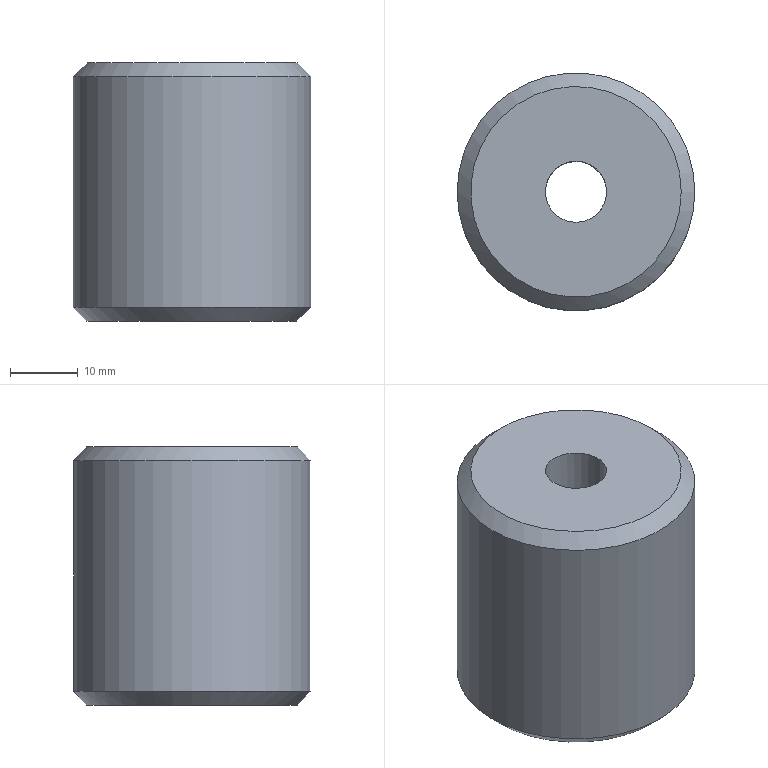Part | STEP file | P011002NM10-000 | 1 solid | 8 faces | box 35 x 35 x 38 mm | volume 32907 mm3 | plane 3 | cylinder 3 | cone 2 | commonest cylinder face diameters 9 x1 14 x1 35 x1
STEP:
#1=CARTESIAN_POINT('',(0.,0.,0.));
#2=DIRECTION('',(0.,0.,1.));
#3=DIRECTION('',(1.,0.,0.));
#4=AXIS2_PLACEMENT_3D('',#1,#2,#3);
#5=CARTESIAN_POINT('',(15.5,100.,-296.));
#6=VERTEX_POINT('',#5);
#7=CARTESIAN_POINT('',(0.,100.,-296.));
#8=DIRECTION('',(0.,0.,1.));
#9=DIRECTION('',(1.,0.,0.));
#10=AXIS2_PLACEMENT_3D('',#7,#8,#9);
#11=CIRCLE('',#10,15.5);
#12=CARTESIAN_POINT('',(0.,100.,-296.));
#13=DIRECTION('',(0.,0.,1.));
#14=DIRECTION('',(1.,0.,0.));
#15=AXIS2_PLACEMENT_3D('',#12,#13,#14);
#16=PLANE('',#15);
#17=CARTESIAN_POINT('',(0.,0.));
#18=DIRECTION('',(1.,0.));
#19=AXIS2_PLACEMENT_2D('',#17,#18);
#20=CIRCLE('',#19,15.5);
#21=(GEOMETRIC_REPRESENTATION_CONTEXT(2)PARAMETRIC_REPRESENTATION_CONTEXT()REPRESENTATION_CONTEXT('',''));
#22=DEFINITIONAL_REPRESENTATION('',(#20),#21);
#23=PCURVE('',#16,#22);
#24=CARTESIAN_POINT('',(0.,100.,-298.));
#25=DIRECTION('',(0.,0.,-1.));
#26=DIRECTION('',(-1.,0.,0.));
#27=AXIS2_PLACEMENT_3D('',#24,#25,#26);
#28=CONICAL_SURFACE('',#27,17.5,0.7854);
#29=CARTESIAN_POINT('',(9.425,-2.));
#30=DIRECTION('',(-1.,0.));
#31=VECTOR('',#30,1.);
#32=LINE('',#29,#31);
#33=(GEOMETRIC_REPRESENTATION_CONTEXT(2)PARAMETRIC_REPRESENTATION_CONTEXT()REPRESENTATION_CONTEXT('',''));
#34=DEFINITIONAL_REPRESENTATION('',(#32),#33);
#35=PCURVE('',#28,#34);
#36=SURFACE_CURVE('',#11,(#23,#35),.PCURVE_S1.);
#37=EDGE_CURVE('',#6,#6,#36,.T.);
#38=ORIENTED_EDGE('',*,*,#37,.T.);
#39=EDGE_LOOP('',(#38));
#40=FACE_BOUND('',#39,.T.);
#41=CARTESIAN_POINT('',(0.,95.5,-296.));
#42=VERTEX_POINT('',#41);
#43=CARTESIAN_POINT('',(0.,100.,-296.));
#44=DIRECTION('',(0.,0.,-1.));
#45=DIRECTION('',(0.,-1.,0.));
#46=AXIS2_PLACEMENT_3D('',#43,#44,#45);
#47=CIRCLE('',#46,4.5);
#48=CARTESIAN_POINT('',(0.,-4.5));
#49=CARTESIAN_POINT('',(-7.794,-4.5));
#50=CARTESIAN_POINT('',(-3.897,2.25));
#51=CARTESIAN_POINT('',(0.,9.));
#52=CARTESIAN_POINT('',(3.897,2.25));
#53=CARTESIAN_POINT('',(7.794,-4.5));
#54=CARTESIAN_POINT('',(0.,-4.5));
#55=(BOUNDED_CURVE()B_SPLINE_CURVE(2,(#48,#49,#50,#51,#52,#53,#54),.UNSPECIFIED.,.T.,.F.)B_SPLINE_CURVE_WITH_KNOTS((1,2,2,2,2,1),(-2.094,0.,2.094,4.189,6.283,8.378),.UNSPECIFIED.)CURVE()GEOMETRIC_REPRESENTATION_ITEM()RATIONAL_B_SPLINE_CURVE((1.,0.5,1.,0.5,1.,0.5,1.))REPRESENTATION_ITEM(''));
#56=(GEOMETRIC_REPRESENTATION_CONTEXT(2)PARAMETRIC_REPRESENTATION_CONTEXT()REPRESENTATION_CONTEXT('',''));
#57=DEFINITIONAL_REPRESENTATION('',(#55),#56);
#58=PCURVE('',#16,#57);
#59=CARTESIAN_POINT('',(0.,100.,-196.848));
#60=DIRECTION('',(0.,0.,-1.));
#61=DIRECTION('',(0.,-1.,0.));
#62=AXIS2_PLACEMENT_3D('',#59,#60,#61);
#63=CYLINDRICAL_SURFACE('',#62,4.5);
#64=CARTESIAN_POINT('',(0.,99.152));
#65=DIRECTION('',(1.,0.));
#66=VECTOR('',#65,1.);
#67=LINE('',#64,#66);
#68=(GEOMETRIC_REPRESENTATION_CONTEXT(2)PARAMETRIC_REPRESENTATION_CONTEXT()REPRESENTATION_CONTEXT('',''));
#69=DEFINITIONAL_REPRESENTATION('',(#67),#68);
#70=PCURVE('',#63,#69);
#71=SURFACE_CURVE('',#47,(#58,#70),.PCURVE_S1.);
#72=EDGE_CURVE('',#42,#42,#71,.T.);
#73=ORIENTED_EDGE('',*,*,#72,.T.);
#74=EDGE_LOOP('',(#73));
#75=FACE_BOUND('',#74,.T.);
#76=ADVANCED_FACE('',(#40,#75),#16,.T.);
#77=CARTESIAN_POINT('',(-17.5,100.,-332.));
#78=VERTEX_POINT('',#77);
#79=CARTESIAN_POINT('',(17.5,100.,-332.));
#80=VERTEX_POINT('',#79);
#81=CARTESIAN_POINT('',(0.,100.,-332.));
#82=DIRECTION('',(0.,0.,1.));
#83=DIRECTION('',(-1.,0.,0.));
#84=AXIS2_PLACEMENT_3D('',#81,#82,#83);
#85=CIRCLE('',#84,17.5);
#86=CARTESIAN_POINT('',(0.,100.,-336.));
#87=DIRECTION('',(0.,0.,1.));
#88=DIRECTION('',(1.,0.,0.));
#89=AXIS2_PLACEMENT_3D('',#86,#87,#88);
#90=CYLINDRICAL_SURFACE('',#89,17.5);
#91=CARTESIAN_POINT('',(3.142,4.));
#92=DIRECTION('',(1.,0.));
#93=VECTOR('',#92,1.);
#94=LINE('',#91,#93);
#95=(GEOMETRIC_REPRESENTATION_CONTEXT(2)PARAMETRIC_REPRESENTATION_CONTEXT()REPRESENTATION_CONTEXT('',''));
#96=DEFINITIONAL_REPRESENTATION('',(#94),#95);
#97=PCURVE('',#90,#96);
#98=CARTESIAN_POINT('',(0.,100.,-332.));
#99=DIRECTION('',(0.,0.,1.));
#100=DIRECTION('',(1.,0.,0.));
#101=AXIS2_PLACEMENT_3D('',#98,#99,#100);
#102=CONICAL_SURFACE('',#101,17.5,0.7854);
#103=CARTESIAN_POINT('',(3.142,0.));
#104=DIRECTION('',(1.,0.));
#105=VECTOR('',#104,1.);
#106=LINE('',#103,#105);
#107=(GEOMETRIC_REPRESENTATION_CONTEXT(2)PARAMETRIC_REPRESENTATION_CONTEXT()REPRESENTATION_CONTEXT('',''));
#108=DEFINITIONAL_REPRESENTATION('',(#106),#107);
#109=PCURVE('',#102,#108);
#110=SURFACE_CURVE('',#85,(#97,#109),.PCURVE_S1.);
#111=EDGE_CURVE('',#78,#80,#110,.T.);
#112=ORIENTED_EDGE('',*,*,#111,.T.);
#113=CARTESIAN_POINT('',(17.5,100.,-298.));
#114=VERTEX_POINT('',#113);
#115=CARTESIAN_POINT('',(17.5,100.,-332.));
#116=CARTESIAN_POINT('',(17.5,100.,-298.));
#117=B_SPLINE_CURVE_WITH_KNOTS('',1,(#115,#116),.UNSPECIFIED.,.F.,.F.,(2,2),(4.,38.),.PIECEWISE_BEZIER_KNOTS.);
#118=CARTESIAN_POINT('',(6.283,0.));
#119=DIRECTION('',(0.,1.));
#120=VECTOR('',#119,1.);
#121=LINE('',#118,#120);
#122=(GEOMETRIC_REPRESENTATION_CONTEXT(2)PARAMETRIC_REPRESENTATION_CONTEXT()REPRESENTATION_CONTEXT('',''));
#123=DEFINITIONAL_REPRESENTATION('',(#121),#122);
#124=PCURVE('',#90,#123);
#125=CARTESIAN_POINT('',(0.,0.));
#126=DIRECTION('',(0.,1.));
#127=VECTOR('',#126,1.);
#128=LINE('',#125,#127);
#129=(GEOMETRIC_REPRESENTATION_CONTEXT(2)PARAMETRIC_REPRESENTATION_CONTEXT()REPRESENTATION_CONTEXT('',''));
#130=DEFINITIONAL_REPRESENTATION('',(#128),#129);
#131=PCURVE('',#90,#130);
#132=SEAM_CURVE('',#117,(#124,#131),.PCURVE_S1.);
#133=EDGE_CURVE('',#80,#114,#132,.T.);
#134=ORIENTED_EDGE('',*,*,#133,.T.);
#135=CARTESIAN_POINT('',(0.,100.,-298.));
#136=DIRECTION('',(0.,0.,-1.));
#137=DIRECTION('',(1.,0.,0.));
#138=AXIS2_PLACEMENT_3D('',#135,#136,#137);
#139=CIRCLE('',#138,17.5);
#140=CARTESIAN_POINT('',(6.283,38.));
#141=DIRECTION('',(-1.,0.));
#142=VECTOR('',#141,1.);
#143=LINE('',#140,#142);
#144=(GEOMETRIC_REPRESENTATION_CONTEXT(2)PARAMETRIC_REPRESENTATION_CONTEXT()REPRESENTATION_CONTEXT('',''));
#145=DEFINITIONAL_REPRESENTATION('',(#143),#144);
#146=PCURVE('',#90,#145);
#147=CARTESIAN_POINT('',(3.142,0.));
#148=DIRECTION('',(1.,0.));
#149=VECTOR('',#148,1.);
#150=LINE('',#147,#149);
#151=(GEOMETRIC_REPRESENTATION_CONTEXT(2)PARAMETRIC_REPRESENTATION_CONTEXT()REPRESENTATION_CONTEXT('',''));
#152=DEFINITIONAL_REPRESENTATION('',(#150),#151);
#153=PCURVE('',#28,#152);
#154=SURFACE_CURVE('',#139,(#146,#153),.PCURVE_S1.);
#155=EDGE_CURVE('',#114,#114,#154,.T.);
#156=ORIENTED_EDGE('',*,*,#155,.T.);
#157=ORIENTED_EDGE('',*,*,#133,.F.);
#158=CARTESIAN_POINT('',(0.,100.,-332.));
#159=DIRECTION('',(0.,0.,1.));
#160=DIRECTION('',(-1.,0.,0.));
#161=AXIS2_PLACEMENT_3D('',#158,#159,#160);
#162=CIRCLE('',#161,17.5);
#163=CARTESIAN_POINT('',(-3.142,4.));
#164=DIRECTION('',(1.,0.));
#165=VECTOR('',#164,1.);
#166=LINE('',#163,#165);
#167=(GEOMETRIC_REPRESENTATION_CONTEXT(2)PARAMETRIC_REPRESENTATION_CONTEXT()REPRESENTATION_CONTEXT('',''));
#168=DEFINITIONAL_REPRESENTATION('',(#166),#167);
#169=PCURVE('',#90,#168);
#170=CARTESIAN_POINT('',(3.142,0.));
#171=DIRECTION('',(1.,0.));
#172=VECTOR('',#171,1.);
#173=LINE('',#170,#172);
#174=(GEOMETRIC_REPRESENTATION_CONTEXT(2)PARAMETRIC_REPRESENTATION_CONTEXT()REPRESENTATION_CONTEXT('',''));
#175=DEFINITIONAL_REPRESENTATION('',(#173),#174);
#176=PCURVE('',#102,#175);
#177=SURFACE_CURVE('',#162,(#169,#176),.PCURVE_S1.);
#178=EDGE_CURVE('',#80,#78,#177,.T.);
#179=ORIENTED_EDGE('',*,*,#178,.T.);
#180=EDGE_LOOP('',(#112,#134,#156,#157,#179));
#181=FACE_BOUND('',#180,.T.);
#182=ADVANCED_FACE('',(#181),#90,.T.);
#183=CARTESIAN_POINT('',(-15.5,100.,-334.));
#184=VERTEX_POINT('',#183);
#185=CARTESIAN_POINT('',(0.,100.,-334.));
#186=DIRECTION('',(0.,0.,-1.));
#187=DIRECTION('',(-1.,0.,0.));
#188=AXIS2_PLACEMENT_3D('',#185,#186,#187);
#189=CIRCLE('',#188,15.5);
#190=CARTESIAN_POINT('',(0.,100.,-334.));
#191=DIRECTION('',(0.,0.,-1.));
#192=DIRECTION('',(-1.,0.,0.));
#193=AXIS2_PLACEMENT_3D('',#190,#191,#192);
#194=PLANE('',#193);
#195=CARTESIAN_POINT('',(0.,0.));
#196=DIRECTION('',(1.,0.));
#197=AXIS2_PLACEMENT_2D('',#195,#196);
#198=CIRCLE('',#197,15.5);
#199=(GEOMETRIC_REPRESENTATION_CONTEXT(2)PARAMETRIC_REPRESENTATION_CONTEXT()REPRESENTATION_CONTEXT('',''));
#200=DEFINITIONAL_REPRESENTATION('',(#198),#199);
#201=PCURVE('',#194,#200);
#202=CARTESIAN_POINT('',(9.425,-2.));
#203=DIRECTION('',(-1.,0.));
#204=VECTOR('',#203,1.);
#205=LINE('',#202,#204);
#206=(GEOMETRIC_REPRESENTATION_CONTEXT(2)PARAMETRIC_REPRESENTATION_CONTEXT()REPRESENTATION_CONTEXT('',''));
#207=DEFINITIONAL_REPRESENTATION('',(#205),#206);
#208=PCURVE('',#102,#207);
#209=SURFACE_CURVE('',#189,(#201,#208),.PCURVE_S1.);
#210=EDGE_CURVE('',#184,#184,#209,.T.);
#211=ORIENTED_EDGE('',*,*,#210,.T.);
#212=EDGE_LOOP('',(#211));
#213=FACE_BOUND('',#212,.T.);
#214=CARTESIAN_POINT('',(0.,93.,-334.));
#215=VERTEX_POINT('',#214);
#216=CARTESIAN_POINT('',(0.,100.,-334.));
#217=DIRECTION('',(0.,0.,-1.));
#218=DIRECTION('',(0.,-1.,0.));
#219=AXIS2_PLACEMENT_3D('',#216,#217,#218);
#220=CIRCLE('',#219,7.);
#221=CARTESIAN_POINT('',(0.,0.));
#222=DIRECTION('',(0.,-1.));
#223=AXIS2_PLACEMENT_2D('',#221,#222);
#224=CIRCLE('',#223,7.);
#225=(GEOMETRIC_REPRESENTATION_CONTEXT(2)PARAMETRIC_REPRESENTATION_CONTEXT()REPRESENTATION_CONTEXT('',''));
#226=DEFINITIONAL_REPRESENTATION('',(#224),#225);
#227=PCURVE('',#194,#226);
#228=CARTESIAN_POINT('',(0.,100.,-194.848));
#229=DIRECTION('',(0.,0.,-1.));
#230=DIRECTION('',(0.,-1.,0.));
#231=AXIS2_PLACEMENT_3D('',#228,#229,#230);
#232=CYLINDRICAL_SURFACE('',#231,7.);
#233=CARTESIAN_POINT('',(0.,139.152));
#234=DIRECTION('',(1.,0.));
#235=VECTOR('',#234,1.);
#236=LINE('',#233,#235);
#237=(GEOMETRIC_REPRESENTATION_CONTEXT(2)PARAMETRIC_REPRESENTATION_CONTEXT()REPRESENTATION_CONTEXT('',''));
#238=DEFINITIONAL_REPRESENTATION('',(#236),#237);
#239=PCURVE('',#232,#238);
#240=SURFACE_CURVE('',#220,(#227,#239),.PCURVE_S1.);
#241=EDGE_CURVE('',#215,#215,#240,.T.);
#242=ORIENTED_EDGE('',*,*,#241,.F.);
#243=EDGE_LOOP('',(#242));
#244=FACE_BOUND('',#243,.T.);
#245=ADVANCED_FACE('',(#213,#244),#194,.T.);
#246=ORIENTED_EDGE('',*,*,#72,.T.);
#247=CARTESIAN_POINT('',(0.,95.5,-325.));
#248=VERTEX_POINT('',#247);
#249=CARTESIAN_POINT('',(0.,95.5,-296.));
#250=CARTESIAN_POINT('',(0.,95.5,-325.));
#251=B_SPLINE_CURVE_WITH_KNOTS('',1,(#249,#250),.UNSPECIFIED.,.F.,.F.,(2,2),(99.152,128.152),.PIECEWISE_BEZIER_KNOTS.);
#252=CARTESIAN_POINT('',(6.283,0.));
#253=DIRECTION('',(0.,1.));
#254=VECTOR('',#253,1.);
#255=LINE('',#252,#254);
#256=(GEOMETRIC_REPRESENTATION_CONTEXT(2)PARAMETRIC_REPRESENTATION_CONTEXT()REPRESENTATION_CONTEXT('',''));
#257=DEFINITIONAL_REPRESENTATION('',(#255),#256);
#258=PCURVE('',#63,#257);
#259=CARTESIAN_POINT('',(0.,0.));
#260=DIRECTION('',(0.,1.));
#261=VECTOR('',#260,1.);
#262=LINE('',#259,#261);
#263=(GEOMETRIC_REPRESENTATION_CONTEXT(2)PARAMETRIC_REPRESENTATION_CONTEXT()REPRESENTATION_CONTEXT('',''));
#264=DEFINITIONAL_REPRESENTATION('',(#262),#263);
#265=PCURVE('',#63,#264);
#266=SEAM_CURVE('',#251,(#258,#265),.PCURVE_S1.);
#267=EDGE_CURVE('',#42,#248,#266,.T.);
#268=ORIENTED_EDGE('',*,*,#267,.T.);
#269=CARTESIAN_POINT('',(-4.5,100.,-325.));
#270=VERTEX_POINT('',#269);
#271=CARTESIAN_POINT('',(0.,100.,-325.));
#272=DIRECTION('',(0.,0.,-1.));
#273=DIRECTION('',(-1.,0.,0.));
#274=AXIS2_PLACEMENT_3D('',#271,#272,#273);
#275=CIRCLE('',#274,4.5);
#276=CARTESIAN_POINT('',(1.571,128.152));
#277=DIRECTION('',(1.,0.));
#278=VECTOR('',#277,1.);
#279=LINE('',#276,#278);
#280=(GEOMETRIC_REPRESENTATION_CONTEXT(2)PARAMETRIC_REPRESENTATION_CONTEXT()REPRESENTATION_CONTEXT('',''));
#281=DEFINITIONAL_REPRESENTATION('',(#279),#280);
#282=PCURVE('',#63,#281);
#283=CARTESIAN_POINT('',(0.,100.,-325.));
#284=DIRECTION('',(0.,0.,-1.));
#285=DIRECTION('',(0.,-1.,0.));
#286=AXIS2_PLACEMENT_3D('',#283,#284,#285);
#287=PLANE('',#286);
#288=CARTESIAN_POINT('',(0.,0.));
#289=DIRECTION('',(0.,1.));
#290=AXIS2_PLACEMENT_2D('',#288,#289);
#291=CIRCLE('',#290,4.5);
#292=(GEOMETRIC_REPRESENTATION_CONTEXT(2)PARAMETRIC_REPRESENTATION_CONTEXT()REPRESENTATION_CONTEXT('',''));
#293=DEFINITIONAL_REPRESENTATION('',(#291),#292);
#294=PCURVE('',#287,#293);
#295=SURFACE_CURVE('',#275,(#282,#294),.PCURVE_S1.);
#296=EDGE_CURVE('',#270,#248,#295,.T.);
#297=ORIENTED_EDGE('',*,*,#296,.F.);
#298=CARTESIAN_POINT('',(0.,100.,-325.));
#299=DIRECTION('',(0.,0.,-1.));
#300=DIRECTION('',(-1.,0.,0.));
#301=AXIS2_PLACEMENT_3D('',#298,#299,#300);
#302=CIRCLE('',#301,4.5);
#303=CARTESIAN_POINT('',(-4.712,128.152));
#304=DIRECTION('',(1.,0.));
#305=VECTOR('',#304,1.);
#306=LINE('',#303,#305);
#307=(GEOMETRIC_REPRESENTATION_CONTEXT(2)PARAMETRIC_REPRESENTATION_CONTEXT()REPRESENTATION_CONTEXT('',''));
#308=DEFINITIONAL_REPRESENTATION('',(#306),#307);
#309=PCURVE('',#63,#308);
#310=CARTESIAN_POINT('',(0.,0.));
#311=DIRECTION('',(0.,1.));
#312=AXIS2_PLACEMENT_2D('',#310,#311);
#313=CIRCLE('',#312,4.5);
#314=(GEOMETRIC_REPRESENTATION_CONTEXT(2)PARAMETRIC_REPRESENTATION_CONTEXT()REPRESENTATION_CONTEXT('',''));
#315=DEFINITIONAL_REPRESENTATION('',(#313),#314);
#316=PCURVE('',#287,#315);
#317=SURFACE_CURVE('',#302,(#309,#316),.PCURVE_S1.);
#318=EDGE_CURVE('',#248,#270,#317,.T.);
#319=ORIENTED_EDGE('',*,*,#318,.F.);
#320=ORIENTED_EDGE('',*,*,#267,.F.);
#321=EDGE_LOOP('',(#246,#268,#297,#319,#320));
#322=FACE_BOUND('',#321,.F.);
#323=ADVANCED_FACE('',(#322),#63,.F.);
#324=CARTESIAN_POINT('',(0.,93.,-325.));
#325=VERTEX_POINT('',#324);
#326=CARTESIAN_POINT('',(0.,100.,-325.));
#327=DIRECTION('',(0.,0.,-1.));
#328=DIRECTION('',(0.,-1.,0.));
#329=AXIS2_PLACEMENT_3D('',#326,#327,#328);
#330=CIRCLE('',#329,7.);
#331=CARTESIAN_POINT('',(0.,0.));
#332=DIRECTION('',(1.,0.));
#333=AXIS2_PLACEMENT_2D('',#331,#332);
#334=CIRCLE('',#333,7.);
#335=(GEOMETRIC_REPRESENTATION_CONTEXT(2)PARAMETRIC_REPRESENTATION_CONTEXT()REPRESENTATION_CONTEXT('',''));
#336=DEFINITIONAL_REPRESENTATION('',(#334),#335);
#337=PCURVE('',#287,#336);
#338=CARTESIAN_POINT('',(0.,130.152));
#339=DIRECTION('',(1.,0.));
#340=VECTOR('',#339,1.);
#341=LINE('',#338,#340);
#342=(GEOMETRIC_REPRESENTATION_CONTEXT(2)PARAMETRIC_REPRESENTATION_CONTEXT()REPRESENTATION_CONTEXT('',''));
#343=DEFINITIONAL_REPRESENTATION('',(#341),#342);
#344=PCURVE('',#232,#343);
#345=SURFACE_CURVE('',#330,(#337,#344),.PCURVE_S1.);
#346=EDGE_CURVE('',#325,#325,#345,.T.);
#347=ORIENTED_EDGE('',*,*,#346,.T.);
#348=EDGE_LOOP('',(#347));
#349=FACE_BOUND('',#348,.T.);
#350=ORIENTED_EDGE('',*,*,#296,.F.);
#351=ORIENTED_EDGE('',*,*,#318,.F.);
#352=EDGE_LOOP('',(#350,#351));
#353=FACE_BOUND('',#352,.T.);
#354=ADVANCED_FACE('',(#349,#353),#287,.T.);
#355=ORIENTED_EDGE('',*,*,#241,.F.);
#356=CARTESIAN_POINT('',(0.,93.,-325.));
#357=CARTESIAN_POINT('',(0.,93.,-334.));
#358=B_SPLINE_CURVE_WITH_KNOTS('',1,(#356,#357),.UNSPECIFIED.,.F.,.F.,(2,2),(130.152,139.152),.PIECEWISE_BEZIER_KNOTS.);
#359=CARTESIAN_POINT('',(0.,0.));
#360=DIRECTION('',(0.,1.));
#361=VECTOR('',#360,1.);
#362=LINE('',#359,#361);
#363=(GEOMETRIC_REPRESENTATION_CONTEXT(2)PARAMETRIC_REPRESENTATION_CONTEXT()REPRESENTATION_CONTEXT('',''));
#364=DEFINITIONAL_REPRESENTATION('',(#362),#363);
#365=PCURVE('',#232,#364);
#366=CARTESIAN_POINT('',(6.283,0.));
#367=DIRECTION('',(0.,1.));
#368=VECTOR('',#367,1.);
#369=LINE('',#366,#368);
#370=(GEOMETRIC_REPRESENTATION_CONTEXT(2)PARAMETRIC_REPRESENTATION_CONTEXT()REPRESENTATION_CONTEXT('',''));
#371=DEFINITIONAL_REPRESENTATION('',(#369),#370);
#372=PCURVE('',#232,#371);
#373=SEAM_CURVE('',#358,(#365,#372),.PCURVE_S1.);
#374=EDGE_CURVE('',#325,#215,#373,.T.);
#375=ORIENTED_EDGE('',*,*,#374,.F.);
#376=ORIENTED_EDGE('',*,*,#346,.T.);
#377=ORIENTED_EDGE('',*,*,#374,.T.);
#378=EDGE_LOOP('',(#355,#375,#376,#377));
#379=FACE_BOUND('',#378,.F.);
#380=ADVANCED_FACE('',(#379),#232,.F.);
#381=ORIENTED_EDGE('',*,*,#210,.F.);
#382=CARTESIAN_POINT('',(-15.5,100.,-334.));
#383=CARTESIAN_POINT('',(-17.5,100.,-332.));
#384=B_SPLINE_CURVE_WITH_KNOTS('',1,(#382,#383),.UNSPECIFIED.,.F.,.F.,(2,2),(-2.828,0.),.PIECEWISE_BEZIER_KNOTS.);
#385=CARTESIAN_POINT('',(9.425,0.));
#386=DIRECTION('',(0.,1.));
#387=VECTOR('',#386,1.);
#388=LINE('',#385,#387);
#389=(GEOMETRIC_REPRESENTATION_CONTEXT(2)PARAMETRIC_REPRESENTATION_CONTEXT()REPRESENTATION_CONTEXT('',''));
#390=DEFINITIONAL_REPRESENTATION('',(#388),#389);
#391=PCURVE('',#102,#390);
#392=CARTESIAN_POINT('',(3.142,0.));
#393=DIRECTION('',(0.,1.));
#394=VECTOR('',#393,1.);
#395=LINE('',#392,#394);
#396=(GEOMETRIC_REPRESENTATION_CONTEXT(2)PARAMETRIC_REPRESENTATION_CONTEXT()REPRESENTATION_CONTEXT('',''));
#397=DEFINITIONAL_REPRESENTATION('',(#395),#396);
#398=PCURVE('',#102,#397);
#399=SEAM_CURVE('',#384,(#391,#398),.PCURVE_S1.);
#400=EDGE_CURVE('',#184,#78,#399,.T.);
#401=ORIENTED_EDGE('',*,*,#400,.T.);
#402=ORIENTED_EDGE('',*,*,#178,.F.);
#403=ORIENTED_EDGE('',*,*,#111,.F.);
#404=ORIENTED_EDGE('',*,*,#400,.F.);
#405=EDGE_LOOP('',(#381,#401,#402,#403,#404));
#406=FACE_BOUND('',#405,.T.);
#407=ADVANCED_FACE('',(#406),#102,.T.);
#408=ORIENTED_EDGE('',*,*,#37,.F.);
#409=CARTESIAN_POINT('',(15.5,100.,-296.));
#410=CARTESIAN_POINT('',(17.5,100.,-298.));
#411=B_SPLINE_CURVE_WITH_KNOTS('',1,(#409,#410),.UNSPECIFIED.,.F.,.F.,(2,2),(-2.828,0.),.PIECEWISE_BEZIER_KNOTS.);
#412=CARTESIAN_POINT('',(9.425,0.));
#413=DIRECTION('',(0.,1.));
#414=VECTOR('',#413,1.);
#415=LINE('',#412,#414);
#416=(GEOMETRIC_REPRESENTATION_CONTEXT(2)PARAMETRIC_REPRESENTATION_CONTEXT()REPRESENTATION_CONTEXT('',''));
#417=DEFINITIONAL_REPRESENTATION('',(#415),#416);
#418=PCURVE('',#28,#417);
#419=CARTESIAN_POINT('',(3.142,0.));
#420=DIRECTION('',(0.,1.));
#421=VECTOR('',#420,1.);
#422=LINE('',#419,#421);
#423=(GEOMETRIC_REPRESENTATION_CONTEXT(2)PARAMETRIC_REPRESENTATION_CONTEXT()REPRESENTATION_CONTEXT('',''));
#424=DEFINITIONAL_REPRESENTATION('',(#422),#423);
#425=PCURVE('',#28,#424);
#426=SEAM_CURVE('',#411,(#418,#425),.PCURVE_S1.);
#427=EDGE_CURVE('',#6,#114,#426,.T.);
#428=ORIENTED_EDGE('',*,*,#427,.T.);
#429=ORIENTED_EDGE('',*,*,#155,.F.);
#430=ORIENTED_EDGE('',*,*,#427,.F.);
#431=EDGE_LOOP('',(#408,#428,#429,#430));
#432=FACE_BOUND('',#431,.T.);
#433=ADVANCED_FACE('',(#432),#28,.T.);
#434=CLOSED_SHELL('',(#76,#182,#245,#323,#354,#380,#407,#433));
#435=MANIFOLD_SOLID_BREP('',#434);
#436=(LENGTH_UNIT()NAMED_UNIT(*)SI_UNIT(.MILLI.,.METRE.));
#437=UNCERTAINTY_MEASURE_WITH_UNIT(LENGTH_MEASURE(0.00001),#436,'','');
#438=(NAMED_UNIT(*)PLANE_ANGLE_UNIT()SI_UNIT($,.RADIAN.));
#439=(NAMED_UNIT(*)SI_UNIT($,.STERADIAN.)SOLID_ANGLE_UNIT());
#440=(GEOMETRIC_REPRESENTATION_CONTEXT(3)GLOBAL_UNCERTAINTY_ASSIGNED_CONTEXT((#437))GLOBAL_UNIT_ASSIGNED_CONTEXT((#436,#438,#439))REPRESENTATION_CONTEXT('',''));
#441=ADVANCED_BREP_SHAPE_REPRESENTATION('',(#4,#435),#440);